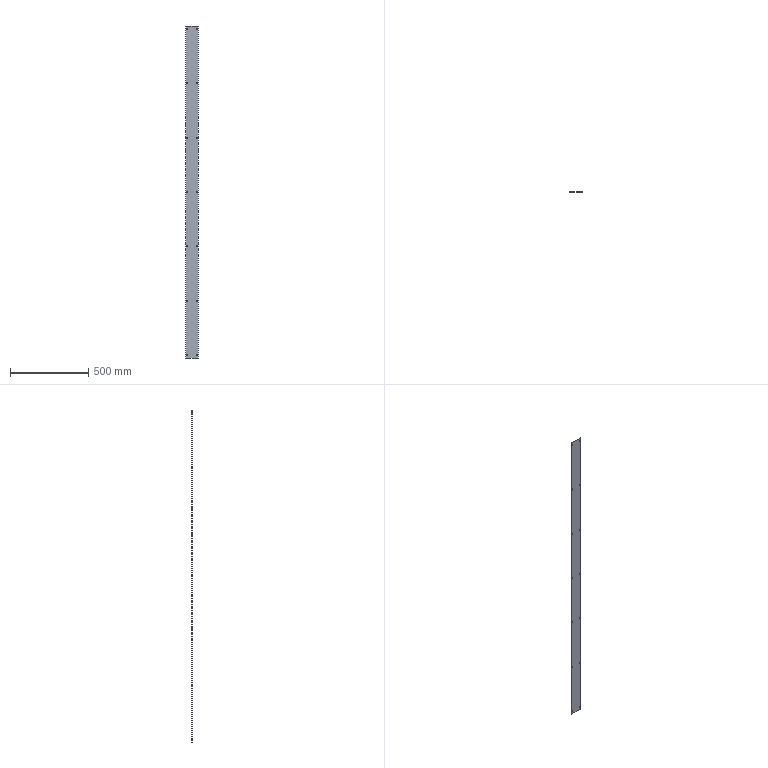Part | SolidWorks | features FlatPattern 1, ICE 1, MirrorPattern 1, SMBaseFlange 1, SheetMetal 1 | 1 solid | 62 faces | box 80 x 1 x 2116 mm | volume 168632 mm3 | plane 34 | cylinder 28 | commonest cylinder face diameters 6 x28